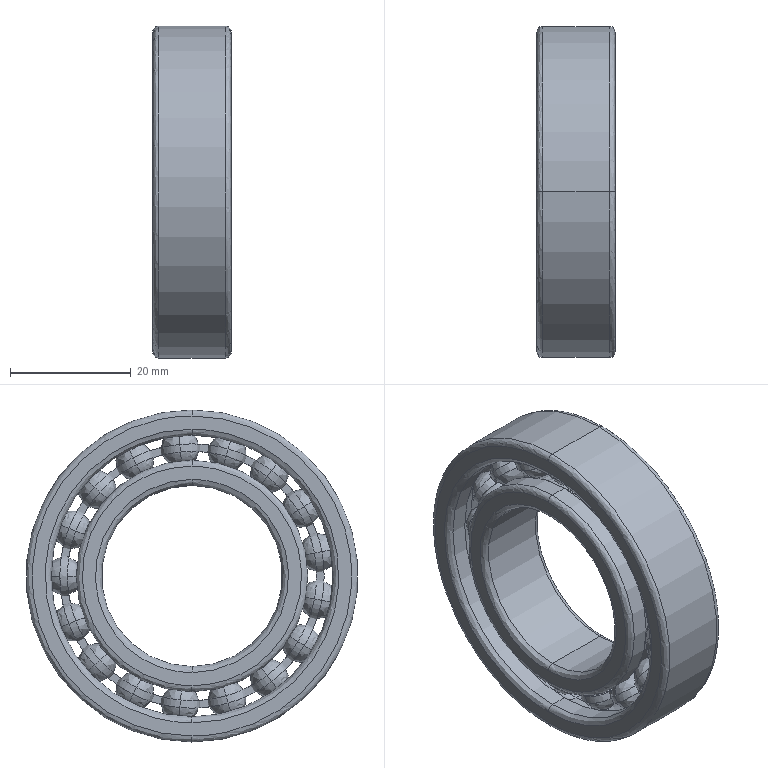Part | SolidWorks | features BaseBody 19 | 19 solids | 209 faces | box 13 x 55 x 55 mm | volume 15839 mm3 | spline 93 | cylinder 78 | plane 38 | commonest cylinder face diameters 41.25 x33 43.75 x33 38.333 x4 46.667 x4 30 x2 55 x2